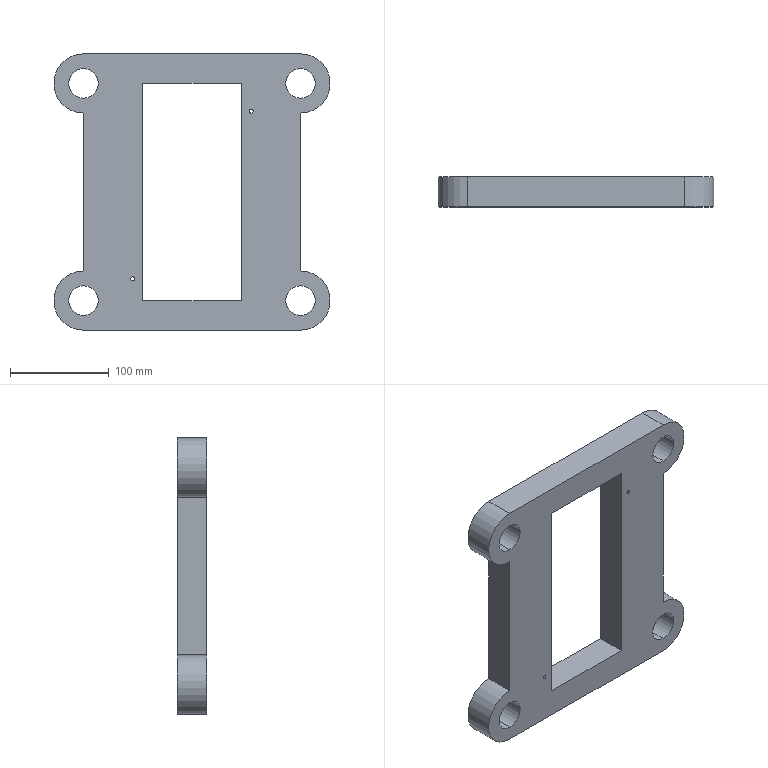Part | SolidWorks | features ICE 2, Extrusion 1, HoleWzd 1, MirrorPattern 1 | 1 solid | 38 faces | box 280 x 30 x 280 mm | volume 1265786 mm3 | cylinder 24 | plane 14 | commonest cylinder face diameters 10 x8 30 x8 4 x4 60 x4
STEP:
#1=CARTESIAN_POINT('',(-60.,0.,19.935));
#2=VERTEX_POINT('',#1);
#3=CARTESIAN_POINT('',(-60.,0.,23.935));
#4=VERTEX_POINT('',#3);
#5=CARTESIAN_POINT('',(-60.,0.,21.935));
#6=DIRECTION('',(0.,1.,0.));
#7=DIRECTION('',(0.,0.,1.));
#8=AXIS2_PLACEMENT_3D('',#5,#6,#7);
#9=CIRCLE('',#8,2.);
#10=EDGE_CURVE('',#2,#4,#9,.T.);
#11=ORIENTED_EDGE('',*,*,#10,.F.);
#12=CARTESIAN_POINT('',(-60.,30.,19.935));
#13=VERTEX_POINT('',#12);
#14=CARTESIAN_POINT('',(-60.,0.,19.935));
#15=DIRECTION('',(0.,1.,0.));
#16=VECTOR('',#15,1000.);
#17=LINE('',#14,#16);
#18=EDGE_CURVE('',#2,#13,#17,.T.);
#19=ORIENTED_EDGE('',*,*,#18,.T.);
#20=CARTESIAN_POINT('',(-60.,30.,23.935));
#21=VERTEX_POINT('',#20);
#22=CARTESIAN_POINT('',(-60.,30.,21.935));
#23=DIRECTION('',(0.,1.,0.));
#24=DIRECTION('',(0.,0.,1.));
#25=AXIS2_PLACEMENT_3D('',#22,#23,#24);
#26=CIRCLE('',#25,2.);
#27=EDGE_CURVE('',#13,#21,#26,.T.);
#28=ORIENTED_EDGE('',*,*,#27,.T.);
#29=CARTESIAN_POINT('',(-60.,0.,23.935));
#30=DIRECTION('',(0.,1.,0.));
#31=VECTOR('',#30,1000.);
#32=LINE('',#29,#31);
#33=EDGE_CURVE('',#4,#21,#32,.T.);
#34=ORIENTED_EDGE('',*,*,#33,.F.);
#35=EDGE_LOOP('',(#11,#19,#28,#34));
#36=FACE_OUTER_BOUND('',#35,.T.);
#37=CARTESIAN_POINT('',(-60.,0.,21.935));
#38=DIRECTION('',(0.,1.,0.));
#39=DIRECTION('',(0.,0.,1.));
#40=AXIS2_PLACEMENT_3D('',#37,#38,#39);
#41=CYLINDRICAL_SURFACE('',#40,2.);
#42=ADVANCED_FACE('',(#36),#41,.F.);
#43=CARTESIAN_POINT('',(60.,0.,189.935));
#44=VERTEX_POINT('',#43);
#45=CARTESIAN_POINT('',(60.,0.,193.935));
#46=VERTEX_POINT('',#45);
#47=CARTESIAN_POINT('',(60.,0.,191.935));
#48=DIRECTION('',(0.,1.,0.));
#49=DIRECTION('',(0.,0.,1.));
#50=AXIS2_PLACEMENT_3D('',#47,#48,#49);
#51=CIRCLE('',#50,2.);
#52=EDGE_CURVE('',#44,#46,#51,.T.);
#53=ORIENTED_EDGE('',*,*,#52,.F.);
#54=CARTESIAN_POINT('',(60.,30.,189.935));
#55=VERTEX_POINT('',#54);
#56=CARTESIAN_POINT('',(60.,0.,189.935));
#57=DIRECTION('',(0.,1.,0.));
#58=VECTOR('',#57,1000.);
#59=LINE('',#56,#58);
#60=EDGE_CURVE('',#44,#55,#59,.T.);
#61=ORIENTED_EDGE('',*,*,#60,.T.);
#62=CARTESIAN_POINT('',(60.,30.,193.935));
#63=VERTEX_POINT('',#62);
#64=CARTESIAN_POINT('',(60.,30.,191.935));
#65=DIRECTION('',(0.,1.,0.));
#66=DIRECTION('',(0.,0.,1.));
#67=AXIS2_PLACEMENT_3D('',#64,#65,#66);
#68=CIRCLE('',#67,2.);
#69=EDGE_CURVE('',#55,#63,#68,.T.);
#70=ORIENTED_EDGE('',*,*,#69,.T.);
#71=CARTESIAN_POINT('',(60.,0.,193.935));
#72=DIRECTION('',(0.,1.,0.));
#73=VECTOR('',#72,1000.);
#74=LINE('',#71,#73);
#75=EDGE_CURVE('',#46,#63,#74,.T.);
#76=ORIENTED_EDGE('',*,*,#75,.F.);
#77=EDGE_LOOP('',(#53,#61,#70,#76));
#78=FACE_OUTER_BOUND('',#77,.T.);
#79=CARTESIAN_POINT('',(60.,0.,191.935));
#80=DIRECTION('',(0.,1.,0.));
#81=DIRECTION('',(0.,0.,1.));
#82=AXIS2_PLACEMENT_3D('',#79,#80,#81);
#83=CYLINDRICAL_SURFACE('',#82,2.);
#84=ADVANCED_FACE('',(#78),#83,.F.);
#85=CARTESIAN_POINT('',(-60.,10.,221.935));
#86=VERTEX_POINT('',#85);
#87=CARTESIAN_POINT('',(-60.,10.,231.935));
#88=VERTEX_POINT('',#87);
#89=CARTESIAN_POINT('',(-60.,10.,226.935));
#90=DIRECTION('',(0.,1.,0.));
#91=DIRECTION('',(0.,0.,1.));
#92=AXIS2_PLACEMENT_3D('',#89,#90,#91);
#93=CIRCLE('',#92,5.);
#94=EDGE_CURVE('',#86,#88,#93,.T.);
#95=ORIENTED_EDGE('',*,*,#94,.F.);
#96=CARTESIAN_POINT('',(-60.,30.,221.935));
#97=VERTEX_POINT('',#96);
#98=CARTESIAN_POINT('',(-60.,10.,221.935));
#99=DIRECTION('',(0.,1.,0.));
#100=VECTOR('',#99,1000.);
#101=LINE('',#98,#100);
#102=EDGE_CURVE('',#86,#97,#101,.T.);
#103=ORIENTED_EDGE('',*,*,#102,.T.);
#104=CARTESIAN_POINT('',(-60.,30.,231.935));
#105=VERTEX_POINT('',#104);
#106=CARTESIAN_POINT('',(-60.,30.,226.935));
#107=DIRECTION('',(0.,1.,0.));
#108=DIRECTION('',(0.,0.,1.));
#109=AXIS2_PLACEMENT_3D('',#106,#107,#108);
#110=CIRCLE('',#109,5.);
#111=EDGE_CURVE('',#97,#105,#110,.T.);
#112=ORIENTED_EDGE('',*,*,#111,.T.);
#113=CARTESIAN_POINT('',(-60.,10.,231.935));
#114=DIRECTION('',(0.,1.,0.));
#115=VECTOR('',#114,1000.);
#116=LINE('',#113,#115);
#117=EDGE_CURVE('',#88,#105,#116,.T.);
#118=ORIENTED_EDGE('',*,*,#117,.F.);
#119=EDGE_LOOP('',(#95,#103,#112,#118));
#120=FACE_OUTER_BOUND('',#119,.T.);
#121=CARTESIAN_POINT('',(-60.,10.,226.935));
#122=DIRECTION('',(0.,1.,0.));
#123=DIRECTION('',(0.,0.,1.));
#124=AXIS2_PLACEMENT_3D('',#121,#122,#123);
#125=CYLINDRICAL_SURFACE('',#124,5.);
#126=ADVANCED_FACE('',(#120),#125,.F.);
#127=CARTESIAN_POINT('',(60.,10.,-18.065));
#128=VERTEX_POINT('',#127);
#129=CARTESIAN_POINT('',(60.,10.,-8.065));
#130=VERTEX_POINT('',#129);
#131=CARTESIAN_POINT('',(60.,10.,-13.065));
#132=DIRECTION('',(0.,1.,0.));
#133=DIRECTION('',(0.,0.,-1.));
#134=AXIS2_PLACEMENT_3D('',#131,#132,#133);
#135=CIRCLE('',#134,5.);
#136=EDGE_CURVE('',#128,#130,#135,.T.);
#137=ORIENTED_EDGE('',*,*,#136,.F.);
#138=CARTESIAN_POINT('',(60.,30.,-18.065));
#139=VERTEX_POINT('',#138);
#140=CARTESIAN_POINT('',(60.,10.,-18.065));
#141=DIRECTION('',(0.,1.,0.));
#142=VECTOR('',#141,1000.);
#143=LINE('',#140,#142);
#144=EDGE_CURVE('',#128,#139,#143,.T.);
#145=ORIENTED_EDGE('',*,*,#144,.T.);
#146=CARTESIAN_POINT('',(60.,30.,-8.065));
#147=VERTEX_POINT('',#146);
#148=CARTESIAN_POINT('',(60.,30.,-13.065));
#149=DIRECTION('',(0.,1.,0.));
#150=DIRECTION('',(0.,0.,-1.));
#151=AXIS2_PLACEMENT_3D('',#148,#149,#150);
#152=CIRCLE('',#151,5.);
#153=EDGE_CURVE('',#139,#147,#152,.T.);
#154=ORIENTED_EDGE('',*,*,#153,.T.);
#155=CARTESIAN_POINT('',(60.,10.,-8.065));
#156=DIRECTION('',(0.,1.,0.));
#157=VECTOR('',#156,1000.);
#158=LINE('',#155,#157);
#159=EDGE_CURVE('',#130,#147,#158,.T.);
#160=ORIENTED_EDGE('',*,*,#159,.F.);
#161=EDGE_LOOP('',(#137,#145,#154,#160));
#162=FACE_OUTER_BOUND('',#161,.T.);
#163=CARTESIAN_POINT('',(60.,10.,-13.065));
#164=DIRECTION('',(0.,1.,0.));
#165=DIRECTION('',(0.,0.,1.));
#166=AXIS2_PLACEMENT_3D('',#163,#164,#165);
#167=CYLINDRICAL_SURFACE('',#166,5.);
#168=ADVANCED_FACE('',(#162),#167,.F.);
#169=CARTESIAN_POINT('',(60.,10.,221.935));
#170=VERTEX_POINT('',#169);
#171=CARTESIAN_POINT('',(60.,10.,231.935));
#172=VERTEX_POINT('',#171);
#173=CARTESIAN_POINT('',(60.,10.,226.935));
#174=DIRECTION('',(0.,1.,0.));
#175=DIRECTION('',(0.,0.,-1.));
#176=AXIS2_PLACEMENT_3D('',#173,#174,#175);
#177=CIRCLE('',#176,5.);
#178=EDGE_CURVE('',#170,#172,#177,.T.);
#179=ORIENTED_EDGE('',*,*,#178,.F.);
#180=CARTESIAN_POINT('',(60.,30.,221.935));
#181=VERTEX_POINT('',#180);
#182=CARTESIAN_POINT('',(60.,10.,221.935));
#183=DIRECTION('',(0.,1.,0.));
#184=VECTOR('',#183,1000.);
#185=LINE('',#182,#184);
#186=EDGE_CURVE('',#170,#181,#185,.T.);
#187=ORIENTED_EDGE('',*,*,#186,.T.);
#188=CARTESIAN_POINT('',(60.,30.,231.935));
#189=VERTEX_POINT('',#188);
#190=CARTESIAN_POINT('',(60.,30.,226.935));
#191=DIRECTION('',(0.,1.,0.));
#192=DIRECTION('',(0.,0.,-1.));
#193=AXIS2_PLACEMENT_3D('',#190,#191,#192);
#194=CIRCLE('',#193,5.);
#195=EDGE_CURVE('',#181,#189,#194,.T.);
#196=ORIENTED_EDGE('',*,*,#195,.T.);
#197=CARTESIAN_POINT('',(60.,10.,231.935));
#198=DIRECTION('',(0.,1.,0.));
#199=VECTOR('',#198,1000.);
#200=LINE('',#197,#199);
#201=EDGE_CURVE('',#172,#189,#200,.T.);
#202=ORIENTED_EDGE('',*,*,#201,.F.);
#203=EDGE_LOOP('',(#179,#187,#196,#202));
#204=FACE_OUTER_BOUND('',#203,.T.);
#205=CARTESIAN_POINT('',(60.,10.,226.935));
#206=DIRECTION('',(0.,1.,0.));
#207=DIRECTION('',(0.,0.,1.));
#208=AXIS2_PLACEMENT_3D('',#205,#206,#207);
#209=CYLINDRICAL_SURFACE('',#208,5.);
#210=ADVANCED_FACE('',(#204),#209,.F.);
#211=CARTESIAN_POINT('',(-60.,10.,-18.065));
#212=VERTEX_POINT('',#211);
#213=CARTESIAN_POINT('',(-60.,10.,-8.065));
#214=VERTEX_POINT('',#213);
#215=CARTESIAN_POINT('',(-60.,10.,-13.065));
#216=DIRECTION('',(0.,1.,0.));
#217=DIRECTION('',(0.,0.,1.));
#218=AXIS2_PLACEMENT_3D('',#215,#216,#217);
#219=CIRCLE('',#218,5.);
#220=EDGE_CURVE('',#212,#214,#219,.T.);
#221=ORIENTED_EDGE('',*,*,#220,.F.);
#222=CARTESIAN_POINT('',(-60.,30.,-18.065));
#223=VERTEX_POINT('',#222);
#224=CARTESIAN_POINT('',(-60.,10.,-18.065));
#225=DIRECTION('',(0.,1.,0.));
#226=VECTOR('',#225,1000.);
#227=LINE('',#224,#226);
#228=EDGE_CURVE('',#212,#223,#227,.T.);
#229=ORIENTED_EDGE('',*,*,#228,.T.);
#230=CARTESIAN_POINT('',(-60.,30.,-8.065));
#231=VERTEX_POINT('',#230);
#232=CARTESIAN_POINT('',(-60.,30.,-13.065));
#233=DIRECTION('',(0.,1.,0.));
#234=DIRECTION('',(0.,0.,1.));
#235=AXIS2_PLACEMENT_3D('',#232,#233,#234);
#236=CIRCLE('',#235,5.);
#237=EDGE_CURVE('',#223,#231,#236,.T.);
#238=ORIENTED_EDGE('',*,*,#237,.T.);
#239=CARTESIAN_POINT('',(-60.,10.,-8.065));
#240=DIRECTION('',(0.,1.,0.));
#241=VECTOR('',#240,1000.);
#242=LINE('',#239,#241);
#243=EDGE_CURVE('',#214,#231,#242,.T.);
#244=ORIENTED_EDGE('',*,*,#243,.F.);
#245=EDGE_LOOP('',(#221,#229,#238,#244));
#246=FACE_OUTER_BOUND('',#245,.T.);
#247=CARTESIAN_POINT('',(-60.,10.,-13.065));
#248=DIRECTION('',(0.,1.,0.));
#249=DIRECTION('',(0.,0.,1.));
#250=AXIS2_PLACEMENT_3D('',#247,#248,#249);
#251=CYLINDRICAL_SURFACE('',#250,5.);
#252=ADVANCED_FACE('',(#246),#251,.F.);
#253=CARTESIAN_POINT('',(110.,30.,235.));
#254=VERTEX_POINT('',#253);
#255=CARTESIAN_POINT('',(110.,30.,205.));
#256=VERTEX_POINT('',#255);
#257=CARTESIAN_POINT('',(110.,30.,220.));
#258=DIRECTION('',(0.,-1.,0.));
#259=DIRECTION('',(0.,0.,1.));
#260=AXIS2_PLACEMENT_3D('',#257,#258,#259);
#261=CIRCLE('',#260,15.);
#262=EDGE_CURVE('',#254,#256,#261,.T.);
#263=ORIENTED_EDGE('',*,*,#262,.F.);
#264=CARTESIAN_POINT('',(110.,0.,235.));
#265=VERTEX_POINT('',#264);
#266=CARTESIAN_POINT('',(110.,30.,235.));
#267=DIRECTION('',(0.,-1.,0.));
#268=VECTOR('',#267,1000.);
#269=LINE('',#266,#268);
#270=EDGE_CURVE('',#254,#265,#269,.T.);
#271=ORIENTED_EDGE('',*,*,#270,.T.);
#272=CARTESIAN_POINT('',(110.,0.,205.));
#273=VERTEX_POINT('',#272);
#274=CARTESIAN_POINT('',(110.,0.,220.));
#275=DIRECTION('',(0.,-1.,0.));
#276=DIRECTION('',(0.,0.,1.));
#277=AXIS2_PLACEMENT_3D('',#274,#275,#276);
#278=CIRCLE('',#277,15.);
#279=EDGE_CURVE('',#265,#273,#278,.T.);
#280=ORIENTED_EDGE('',*,*,#279,.T.);
#281=CARTESIAN_POINT('',(110.,30.,205.));
#282=DIRECTION('',(0.,-1.,0.));
#283=VECTOR('',#282,1000.);
#284=LINE('',#281,#283);
#285=EDGE_CURVE('',#256,#273,#284,.T.);
#286=ORIENTED_EDGE('',*,*,#285,.F.);
#287=EDGE_LOOP('',(#263,#271,#280,#286));
#288=FACE_OUTER_BOUND('',#287,.T.);
#289=CARTESIAN_POINT('',(110.,30.,220.));
#290=DIRECTION('',(0.,-1.,0.));
#291=DIRECTION('',(0.,0.,-1.));
#292=AXIS2_PLACEMENT_3D('',#289,#290,#291);
#293=CYLINDRICAL_SURFACE('',#292,15.);
#294=ADVANCED_FACE('',(#288),#293,.F.);
#295=CARTESIAN_POINT('',(110.,30.,15.));
#296=VERTEX_POINT('',#295);
#297=CARTESIAN_POINT('',(110.,30.,-15.));
#298=VERTEX_POINT('',#297);
#299=CARTESIAN_POINT('',(110.,30.,0.));
#300=DIRECTION('',(0.,-1.,0.));
#301=DIRECTION('',(0.,0.,1.));
#302=AXIS2_PLACEMENT_3D('',#299,#300,#301);
#303=CIRCLE('',#302,15.);
#304=EDGE_CURVE('',#296,#298,#303,.T.);
#305=ORIENTED_EDGE('',*,*,#304,.F.);
#306=CARTESIAN_POINT('',(110.,0.,15.));
#307=VERTEX_POINT('',#306);
#308=CARTESIAN_POINT('',(110.,30.,15.));
#309=DIRECTION('',(0.,-1.,0.));
#310=VECTOR('',#309,1000.);
#311=LINE('',#308,#310);
#312=EDGE_CURVE('',#296,#307,#311,.T.);
#313=ORIENTED_EDGE('',*,*,#312,.T.);
#314=CARTESIAN_POINT('',(110.,0.,-15.));
#315=VERTEX_POINT('',#314);
#316=CARTESIAN_POINT('',(110.,0.,0.));
#317=DIRECTION('',(0.,-1.,0.));
#318=DIRECTION('',(0.,0.,1.));
#319=AXIS2_PLACEMENT_3D('',#316,#317,#318);
#320=CIRCLE('',#319,15.);
#321=EDGE_CURVE('',#307,#315,#320,.T.);
#322=ORIENTED_EDGE('',*,*,#321,.T.);
#323=CARTESIAN_POINT('',(110.,30.,-15.));
#324=DIRECTION('',(0.,-1.,0.));
#325=VECTOR('',#324,1000.);
#326=LINE('',#323,#325);
#327=EDGE_CURVE('',#298,#315,#326,.T.);
#328=ORIENTED_EDGE('',*,*,#327,.F.);
#329=EDGE_LOOP('',(#305,#313,#322,#328));
#330=FACE_OUTER_BOUND('',#329,.T.);
#331=CARTESIAN_POINT('',(110.,30.,0.));
#332=DIRECTION('',(0.,-1.,0.));
#333=DIRECTION('',(0.,0.,-1.));
#334=AXIS2_PLACEMENT_3D('',#331,#332,#333);
#335=CYLINDRICAL_SURFACE('',#334,15.);
#336=ADVANCED_FACE('',(#330),#335,.F.);
#337=CARTESIAN_POINT('',(-110.,30.,205.));
#338=VERTEX_POINT('',#337);
#339=CARTESIAN_POINT('',(-110.,30.,235.));
#340=VERTEX_POINT('',#339);
#341=CARTESIAN_POINT('',(-110.,30.,220.));
#342=DIRECTION('',(0.,1.,0.));
#343=DIRECTION('',(0.,0.,1.));
#344=AXIS2_PLACEMENT_3D('',#341,#342,#343);
#345=CIRCLE('',#344,15.);
#346=EDGE_CURVE('',#338,#340,#345,.T.);
#347=ORIENTED_EDGE('',*,*,#346,.T.);
#348=CARTESIAN_POINT('',(-110.,0.,235.));
#349=VERTEX_POINT('',#348);
#350=CARTESIAN_POINT('',(-110.,30.,235.));
#351=DIRECTION('',(0.,-1.,0.));
#352=VECTOR('',#351,1000.);
#353=LINE('',#350,#352);
#354=EDGE_CURVE('',#340,#349,#353,.T.);
#355=ORIENTED_EDGE('',*,*,#354,.T.);
#356=CARTESIAN_POINT('',(-110.,0.,205.));
#357=VERTEX_POINT('',#356);
#358=CARTESIAN_POINT('',(-110.,0.,220.));
#359=DIRECTION('',(0.,1.,0.));
#360=DIRECTION('',(0.,0.,1.));
#361=AXIS2_PLACEMENT_3D('',#358,#359,#360);
#362=CIRCLE('',#361,15.);
#363=EDGE_CURVE('',#357,#349,#362,.T.);
#364=ORIENTED_EDGE('',*,*,#363,.F.);
#365=CARTESIAN_POINT('',(-110.,30.,205.));
#366=DIRECTION('',(0.,-1.,0.));
#367=VECTOR('',#366,1000.);
#368=LINE('',#365,#367);
#369=EDGE_CURVE('',#338,#357,#368,.T.);
#370=ORIENTED_EDGE('',*,*,#369,.F.);
#371=EDGE_LOOP('',(#347,#355,#364,#370));
#372=FACE_OUTER_BOUND('',#371,.T.);
#373=CARTESIAN_POINT('',(-110.,30.,220.));
#374=DIRECTION('',(0.,-1.,0.));
#375=DIRECTION('',(0.,0.,-1.));
#376=AXIS2_PLACEMENT_3D('',#373,#374,#375);
#377=CYLINDRICAL_SURFACE('',#376,15.);
#378=ADVANCED_FACE('',(#372),#377,.F.);
#379=CARTESIAN_POINT('',(-110.,30.,-15.));
#380=VERTEX_POINT('',#379);
#381=CARTESIAN_POINT('',(-110.,30.,15.));
#382=VERTEX_POINT('',#381);
#383=CARTESIAN_POINT('',(-110.,30.,0.));
#384=DIRECTION('',(0.,1.,0.));
#385=DIRECTION('',(0.,0.,1.));
#386=AXIS2_PLACEMENT_3D('',#383,#384,#385);
#387=CIRCLE('',#386,15.);
#388=EDGE_CURVE('',#380,#382,#387,.T.);
#389=ORIENTED_EDGE('',*,*,#388,.T.);
#390=CARTESIAN_POINT('',(-110.,0.,15.));
#391=VERTEX_POINT('',#390);
#392=CARTESIAN_POINT('',(-110.,30.,15.));
#393=DIRECTION('',(0.,-1.,0.));
#394=VECTOR('',#393,1000.);
#395=LINE('',#392,#394);
#396=EDGE_CURVE('',#382,#391,#395,.T.);
#397=ORIENTED_EDGE('',*,*,#396,.T.);
#398=CARTESIAN_POINT('',(-110.,0.,-15.));
#399=VERTEX_POINT('',#398);
#400=CARTESIAN_POINT('',(-110.,0.,0.));
#401=DIRECTION('',(0.,1.,0.));
#402=DIRECTION('',(0.,0.,1.));
#403=AXIS2_PLACEMENT_3D('',#400,#401,#402);
#404=CIRCLE('',#403,15.);
#405=EDGE_CURVE('',#399,#391,#404,.T.);
#406=ORIENTED_EDGE('',*,*,#405,.F.);
#407=CARTESIAN_POINT('',(-110.,30.,-15.));
#408=DIRECTION('',(0.,-1.,0.));
#409=VECTOR('',#408,1000.);
#410=LINE('',#407,#409);
#411=EDGE_CURVE('',#380,#399,#410,.T.);
#412=ORIENTED_EDGE('',*,*,#411,.F.);
#413=EDGE_LOOP('',(#389,#397,#406,#412));
#414=FACE_OUTER_BOUND('',#413,.T.);
#415=CARTESIAN_POINT('',(-110.,30.,0.));
#416=DIRECTION('',(0.,-1.,0.));
#417=DIRECTION('',(0.,0.,-1.));
#418=AXIS2_PLACEMENT_3D('',#415,#416,#417);
#419=CYLINDRICAL_SURFACE('',#418,15.);
#420=ADVANCED_FACE('',(#414),#419,.F.);
#421=CARTESIAN_POINT('',(-60.,30.,21.935));
#422=DIRECTION('',(0.,1.,0.));
#423=DIRECTION('',(0.,0.,1.));
#424=AXIS2_PLACEMENT_3D('',#421,#422,#423);
#425=CIRCLE('',#424,2.);
#426=EDGE_CURVE('',#21,#13,#425,.T.);
#427=ORIENTED_EDGE('',*,*,#426,.F.);
#428=ORIENTED_EDGE('',*,*,#27,.F.);
#429=EDGE_LOOP('',(#427,#428));
#430=FACE_BOUND('',#429,.T.);
#431=CARTESIAN_POINT('',(60.,30.,191.935));
#432=DIRECTION('',(0.,1.,0.));
#433=DIRECTION('',(0.,0.,1.));
#434=AXIS2_PLACEMENT_3D('',#431,#432,#433);
#435=CIRCLE('',#434,2.);
#436=EDGE_CURVE('',#63,#55,#435,.T.);
#437=ORIENTED_EDGE('',*,*,#436,.F.);
#438=ORIENTED_EDGE('',*,*,#69,.F.);
#439=EDGE_LOOP('',(#437,#438));
#440=FACE_BOUND('',#439,.T.);
#441=CARTESIAN_POINT('',(-60.,30.,226.935));
#442=DIRECTION('',(0.,1.,0.));
#443=DIRECTION('',(0.,0.,1.));
#444=AXIS2_PLACEMENT_3D('',#441,#442,#443);
#445=CIRCLE('',#444,5.);
#446=EDGE_CURVE('',#105,#97,#445,.T.);
#447=ORIENTED_EDGE('',*,*,#446,.F.);
#448=ORIENTED_EDGE('',*,*,#111,.F.);
#449=EDGE_LOOP('',(#447,#448));
#450=FACE_BOUND('',#449,.T.);
#451=CARTESIAN_POINT('',(60.,30.,-13.065));
#452=DIRECTION('',(0.,1.,0.));
#453=DIRECTION('',(0.,0.,-1.));
#454=AXIS2_PLACEMENT_3D('',#451,#452,#453);
#455=CIRCLE('',#454,5.);
#456=EDGE_CURVE('',#147,#139,#455,.T.);
#457=ORIENTED_EDGE('',*,*,#456,.F.);
#458=ORIENTED_EDGE('',*,*,#153,.F.);
#459=EDGE_LOOP('',(#457,#458));
#460=FACE_BOUND('',#459,.T.);
#461=CARTESIAN_POINT('',(60.,30.,226.935));
#462=DIRECTION('',(0.,1.,0.));
#463=DIRECTION('',(0.,0.,-1.));
#464=AXIS2_PLACEMENT_3D('',#461,#462,#463);
#465=CIRCLE('',#464,5.);
#466=EDGE_CURVE('',#189,#181,#465,.T.);
#467=ORIENTED_EDGE('',*,*,#466,.F.);
#468=ORIENTED_EDGE('',*,*,#195,.F.);
#469=EDGE_LOOP('',(#467,#468));
#470=FACE_BOUND('',#469,.T.);
#471=CARTESIAN_POINT('',(-60.,30.,-13.065));
#472=DIRECTION('',(0.,1.,0.));
#473=DIRECTION('',(0.,0.,1.));
#474=AXIS2_PLACEMENT_3D('',#471,#472,#473);
#475=CIRCLE('',#474,5.);
#476=EDGE_CURVE('',#231,#223,#475,.T.);
#477=ORIENTED_EDGE('',*,*,#476,.F.);
#478=ORIENTED_EDGE('',*,*,#237,.F.);
#479=EDGE_LOOP('',(#477,#478));
#480=FACE_BOUND('',#479,.T.);
#481=CARTESIAN_POINT('',(-110.,30.,250.));
#482=VERTEX_POINT('',#481);
#483=CARTESIAN_POINT('',(110.,30.,250.));
#484=VERTEX_POINT('',#483);
#485=CARTESIAN_POINT('',(-110.,30.,250.));
#486=DIRECTION('',(1.,0.,0.));
#487=VECTOR('',#486,1000.);
#488=LINE('',#485,#487);
#489=EDGE_CURVE('',#482,#484,#488,.T.);
#490=ORIENTED_EDGE('',*,*,#489,.T.);
#491=CARTESIAN_POINT('',(110.,30.,190.));
#492=VERTEX_POINT('',#491);
#493=CARTESIAN_POINT('',(110.,30.,220.));
#494=DIRECTION('',(0.,-1.,0.));
#495=DIRECTION('',(0.,0.,1.));
#496=AXIS2_PLACEMENT_3D('',#493,#494,#495);
#497=CIRCLE('',#496,30.);
#498=EDGE_CURVE('',#492,#484,#497,.T.);
#499=ORIENTED_EDGE('',*,*,#498,.F.);
#500=CARTESIAN_POINT('',(110.,30.,30.));
#501=VERTEX_POINT('',#500);
#502=CARTESIAN_POINT('',(110.,30.,190.));
#503=DIRECTION('',(0.,0.,1.));
#504=VECTOR('',#503,1000.);
#505=LINE('',#502,#504);
#506=EDGE_CURVE('',#501,#492,#505,.T.);
#507=ORIENTED_EDGE('',*,*,#506,.F.);
#508=CARTESIAN_POINT('',(110.,30.,-30.));
#509=VERTEX_POINT('',#508);
#510=CARTESIAN_POINT('',(110.,30.,0.));
#511=DIRECTION('',(0.,-1.,0.));
#512=DIRECTION('',(0.,0.,1.));
#513=AXIS2_PLACEMENT_3D('',#510,#511,#512);
#514=CIRCLE('',#513,30.);
#515=EDGE_CURVE('',#509,#501,#514,.T.);
#516=ORIENTED_EDGE('',*,*,#515,.F.);
#517=CARTESIAN_POINT('',(-110.,30.,-30.));
#518=VERTEX_POINT('',#517);
#519=CARTESIAN_POINT('',(80.,30.,-30.));
#520=DIRECTION('',(-1.,0.,0.));
#521=VECTOR('',#520,1000.);
#522=LINE('',#519,#521);
#523=EDGE_CURVE('',#509,#518,#522,.T.);
#524=ORIENTED_EDGE('',*,*,#523,.T.);
#525=CARTESIAN_POINT('',(-110.,30.,30.));
#526=VERTEX_POINT('',#525);
#527=CARTESIAN_POINT('',(-110.,30.,0.));
#528=DIRECTION('',(0.,1.,0.));
#529=DIRECTION('',(0.,0.,1.));
#530=AXIS2_PLACEMENT_3D('',#527,#528,#529);
#531=CIRCLE('',#530,30.);
#532=EDGE_CURVE('',#518,#526,#531,.T.);
#533=ORIENTED_EDGE('',*,*,#532,.T.);
#534=CARTESIAN_POINT('',(-110.,30.,190.));
#535=VERTEX_POINT('',#534);
#536=CARTESIAN_POINT('',(-110.,30.,190.));
#537=DIRECTION('',(0.,0.,1.));
#538=VECTOR('',#537,1000.);
#539=LINE('',#536,#538);
#540=EDGE_CURVE('',#526,#535,#539,.T.);
#541=ORIENTED_EDGE('',*,*,#540,.T.);
#542=CARTESIAN_POINT('',(-110.,30.,220.));
#543=DIRECTION('',(0.,1.,0.));
#544=DIRECTION('',(0.,0.,1.));
#545=AXIS2_PLACEMENT_3D('',#542,#543,#544);
#546=CIRCLE('',#545,30.);
#547=EDGE_CURVE('',#535,#482,#546,.T.);
#548=ORIENTED_EDGE('',*,*,#547,.T.);
#549=EDGE_LOOP('',(#490,#499,#507,#516,#524,#533,#541,#548));
#550=FACE_OUTER_BOUND('',#549,.T.);
#551=ORIENTED_EDGE('',*,*,#388,.F.);
#552=CARTESIAN_POINT('',(-110.,30.,0.));
#553=DIRECTION('',(0.,1.,0.));
#554=DIRECTION('',(0.,0.,1.));
#555=AXIS2_PLACEMENT_3D('',#552,#553,#554);
#556=CIRCLE('',#555,15.);
#557=EDGE_CURVE('',#382,#380,#556,.T.);
#558=ORIENTED_EDGE('',*,*,#557,.F.);
#559=EDGE_LOOP('',(#551,#558));
#560=FACE_BOUND('',#559,.T.);
#561=ORIENTED_EDGE('',*,*,#346,.F.);
#562=CARTESIAN_POINT('',(-110.,30.,220.));
#563=DIRECTION('',(0.,1.,0.));
#564=DIRECTION('',(0.,0.,1.));
#565=AXIS2_PLACEMENT_3D('',#562,#563,#564);
#566=CIRCLE('',#565,15.);
#567=EDGE_CURVE('',#340,#338,#566,.T.);
#568=ORIENTED_EDGE('',*,*,#567,.F.);
#569=EDGE_LOOP('',(#561,#568));
#570=FACE_BOUND('',#569,.T.);
#571=CARTESIAN_POINT('',(-50.,30.,0.));
#572=VERTEX_POINT('',#571);
#573=CARTESIAN_POINT('',(-50.,30.,220.));
#574=VERTEX_POINT('',#573);
#575=CARTESIAN_POINT('',(-50.,30.,0.));
#576=DIRECTION('',(0.,0.,1.));
#577=VECTOR('',#576,1000.);
#578=LINE('',#575,#577);
#579=EDGE_CURVE('',#572,#574,#578,.T.);
#580=ORIENTED_EDGE('',*,*,#579,.F.);
#581=CARTESIAN_POINT('',(50.,30.,0.));
#582=VERTEX_POINT('',#581);
#583=CARTESIAN_POINT('',(50.,30.,0.));
#584=DIRECTION('',(-1.,0.,0.));
#585=VECTOR('',#584,1000.);
#586=LINE('',#583,#585);
#587=EDGE_CURVE('',#582,#572,#586,.T.);
#588=ORIENTED_EDGE('',*,*,#587,.F.);
#589=CARTESIAN_POINT('',(50.,30.,220.));
#590=VERTEX_POINT('',#589);
#591=CARTESIAN_POINT('',(50.,30.,220.));
#592=DIRECTION('',(0.,0.,-1.));
#593=VECTOR('',#592,1000.);
#594=LINE('',#591,#593);
#595=EDGE_CURVE('',#590,#582,#594,.T.);
#596=ORIENTED_EDGE('',*,*,#595,.F.);
#597=CARTESIAN_POINT('',(-50.,30.,220.));
#598=DIRECTION('',(1.,0.,0.));
#599=VECTOR('',#598,1000.);
#600=LINE('',#597,#599);
#601=EDGE_CURVE('',#574,#590,#600,.T.);
#602=ORIENTED_EDGE('',*,*,#601,.F.);
#603=EDGE_LOOP('',(#580,#588,#596,#602));
#604=FACE_BOUND('',#603,.T.);
#605=CARTESIAN_POINT('',(110.,30.,0.));
#606=DIRECTION('',(0.,-1.,0.));
#607=DIRECTION('',(0.,0.,1.));
#608=AXIS2_PLACEMENT_3D('',#605,#606,#607);
#609=CIRCLE('',#608,15.);
#610=EDGE_CURVE('',#298,#296,#609,.T.);
#611=ORIENTED_EDGE('',*,*,#610,.T.);
#612=ORIENTED_EDGE('',*,*,#304,.T.);
#613=EDGE_LOOP('',(#611,#612));
#614=FACE_BOUND('',#613,.T.);
#615=CARTESIAN_POINT('',(110.,30.,220.));
#616=DIRECTION('',(0.,-1.,0.));
#617=DIRECTION('',(0.,0.,1.));
#618=AXIS2_PLACEMENT_3D('',#615,#616,#617);
#619=CIRCLE('',#618,15.);
#620=EDGE_CURVE('',#256,#254,#619,.T.);
#621=ORIENTED_EDGE('',*,*,#620,.T.);
#622=ORIENTED_EDGE('',*,*,#262,.T.);
#623=EDGE_LOOP('',(#621,#622));
#624=FACE_BOUND('',#623,.T.);
#625=CARTESIAN_POINT('',(-110.,30.,0.));
#626=DIRECTION('',(0.,1.,0.));
#627=DIRECTION('',(0.,0.,1.));
#628=AXIS2_PLACEMENT_3D('',#625,#626,#627);
#629=PLANE('',#628);
#630=ADVANCED_FACE('',(#430,#440,#450,#460,#470,#480,#550,#560,#570,#604,#614,#624),#629,.T.);
#631=CARTESIAN_POINT('',(-60.,0.,21.935));
#632=DIRECTION('',(0.,1.,0.));
#633=DIRECTION('',(0.,0.,1.));
#634=AXIS2_PLACEMENT_3D('',#631,#632,#633);
#635=CIRCLE('',#634,2.);
#636=EDGE_CURVE('',#4,#2,#635,.T.);
#637=ORIENTED_EDGE('',*,*,#636,.T.);
#638=ORIENTED_EDGE('',*,*,#10,.T.);
#639=EDGE_LOOP('',(#637,#638));
#640=FACE_BOUND('',#639,.T.);
#641=CARTESIAN_POINT('',(60.,0.,191.935));
#642=DIRECTION('',(0.,1.,0.));
#643=DIRECTION('',(0.,0.,1.));
#644=AXIS2_PLACEMENT_3D('',#641,#642,#643);
#645=CIRCLE('',#644,2.);
#646=EDGE_CURVE('',#46,#44,#645,.T.);
#647=ORIENTED_EDGE('',*,*,#646,.T.);
#648=ORIENTED_EDGE('',*,*,#52,.T.);
#649=EDGE_LOOP('',(#647,#648));
#650=FACE_BOUND('',#649,.T.);
#651=ORIENTED_EDGE('',*,*,#405,.T.);
#652=CARTESIAN_POINT('',(-110.,0.,0.));
#653=DIRECTION('',(0.,1.,0.));
#654=DIRECTION('',(0.,0.,1.));
#655=AXIS2_PLACEMENT_3D('',#652,#653,#654);
#656=CIRCLE('',#655,15.);
#657=EDGE_CURVE('',#391,#399,#656,.T.);
#658=ORIENTED_EDGE('',*,*,#657,.T.);
#659=EDGE_LOOP('',(#651,#658));
#660=FACE_BOUND('',#659,.T.);
#661=CARTESIAN_POINT('',(-110.,0.,-30.));
#662=VERTEX_POINT('',#661);
#663=CARTESIAN_POINT('',(-110.,0.,30.));
#664=VERTEX_POINT('',#663);
#665=CARTESIAN_POINT('',(-110.,0.,0.));
#666=DIRECTION('',(0.,1.,0.));
#667=DIRECTION('',(0.,0.,1.));
#668=AXIS2_PLACEMENT_3D('',#665,#666,#667);
#669=CIRCLE('',#668,30.);
#670=EDGE_CURVE('',#662,#664,#669,.T.);
#671=ORIENTED_EDGE('',*,*,#670,.F.);
#672=CARTESIAN_POINT('',(110.,0.,-30.));
#673=VERTEX_POINT('',#672);
#674=CARTESIAN_POINT('',(80.,0.,-30.));
#675=DIRECTION('',(-1.,0.,0.));
#676=VECTOR('',#675,1000.);
#677=LINE('',#674,#676);
#678=EDGE_CURVE('',#673,#662,#677,.T.);
#679=ORIENTED_EDGE('',*,*,#678,.F.);
#680=CARTESIAN_POINT('',(110.,0.,30.));
#681=VERTEX_POINT('',#680);
#682=CARTESIAN_POINT('',(110.,0.,0.));
#683=DIRECTION('',(0.,-1.,0.));
#684=DIRECTION('',(0.,0.,1.));
#685=AXIS2_PLACEMENT_3D('',#682,#683,#684);
#686=CIRCLE('',#685,30.);
#687=EDGE_CURVE('',#673,#681,#686,.T.);
#688=ORIENTED_EDGE('',*,*,#687,.T.);
#689=CARTESIAN_POINT('',(110.,0.,190.));
#690=VERTEX_POINT('',#689);
#691=CARTESIAN_POINT('',(110.,0.,190.));
#692=DIRECTION('',(0.,0.,1.));
#693=VECTOR('',#692,1000.);
#694=LINE('',#691,#693);
#695=EDGE_CURVE('',#681,#690,#694,.T.);
#696=ORIENTED_EDGE('',*,*,#695,.T.);
#697=CARTESIAN_POINT('',(110.,0.,250.));
#698=VERTEX_POINT('',#697);
#699=CARTESIAN_POINT('',(110.,0.,220.));
#700=DIRECTION('',(0.,-1.,0.));
#701=DIRECTION('',(0.,0.,1.));
#702=AXIS2_PLACEMENT_3D('',#699,#700,#701);
#703=CIRCLE('',#702,30.);
#704=EDGE_CURVE('',#690,#698,#703,.T.);
#705=ORIENTED_EDGE('',*,*,#704,.T.);
#706=CARTESIAN_POINT('',(-110.,0.,250.));
#707=VERTEX_POINT('',#706);
#708=CARTESIAN_POINT('',(-110.,0.,250.));
#709=DIRECTION('',(1.,0.,0.));
#710=VECTOR('',#709,1000.);
#711=LINE('',#708,#710);
#712=EDGE_CURVE('',#707,#698,#711,.T.);
#713=ORIENTED_EDGE('',*,*,#712,.F.);
#714=CARTESIAN_POINT('',(-110.,0.,190.));
#715=VERTEX_POINT('',#714);
#716=CARTESIAN_POINT('',(-110.,0.,220.));
#717=DIRECTION('',(0.,1.,0.));
#718=DIRECTION('',(0.,0.,1.));
#719=AXIS2_PLACEMENT_3D('',#716,#717,#718);
#720=CIRCLE('',#719,30.);
#721=EDGE_CURVE('',#715,#707,#720,.T.);
#722=ORIENTED_EDGE('',*,*,#721,.F.);
#723=CARTESIAN_POINT('',(-110.,0.,190.));
#724=DIRECTION('',(0.,0.,1.));
#725=VECTOR('',#724,1000.);
#726=LINE('',#723,#725);
#727=EDGE_CURVE('',#664,#715,#726,.T.);
#728=ORIENTED_EDGE('',*,*,#727,.F.);
#729=EDGE_LOOP('',(#671,#679,#688,#696,#705,#713,#722,#728));
#730=FACE_OUTER_BOUND('',#729,.T.);
#731=ORIENTED_EDGE('',*,*,#363,.T.);
#732=CARTESIAN_POINT('',(-110.,0.,220.));
#733=DIRECTION('',(0.,1.,0.));
#734=DIRECTION('',(0.,0.,1.));
#735=AXIS2_PLACEMENT_3D('',#732,#733,#734);
#736=CIRCLE('',#735,15.);
#737=EDGE_CURVE('',#349,#357,#736,.T.);
#738=ORIENTED_EDGE('',*,*,#737,.T.);
#739=EDGE_LOOP('',(#731,#738));
#740=FACE_BOUND('',#739,.T.);
#741=CARTESIAN_POINT('',(50.,0.,0.));
#742=VERTEX_POINT('',#741);
#743=CARTESIAN_POINT('',(-50.,0.,0.));
#744=VERTEX_POINT('',#743);
#745=CARTESIAN_POINT('',(50.,0.,0.));
#746=DIRECTION('',(-1.,0.,0.));
#747=VECTOR('',#746,1000.);
#748=LINE('',#745,#747);
#749=EDGE_CURVE('',#742,#744,#748,.T.);
#750=ORIENTED_EDGE('',*,*,#749,.T.);
#751=CARTESIAN_POINT('',(-50.,0.,220.));
#752=VERTEX_POINT('',#751);
#753=CARTESIAN_POINT('',(-50.,0.,0.));
#754=DIRECTION('',(0.,0.,1.));
#755=VECTOR('',#754,1000.);
#756=LINE('',#753,#755);
#757=EDGE_CURVE('',#744,#752,#756,.T.);
#758=ORIENTED_EDGE('',*,*,#757,.T.);
#759=CARTESIAN_POINT('',(50.,0.,220.));
#760=VERTEX_POINT('',#759);
#761=CARTESIAN_POINT('',(-50.,0.,220.));
#762=DIRECTION('',(1.,0.,0.));
#763=VECTOR('',#762,1000.);
#764=LINE('',#761,#763);
#765=EDGE_CURVE('',#752,#760,#764,.T.);
#766=ORIENTED_EDGE('',*,*,#765,.T.);
#767=CARTESIAN_POINT('',(50.,0.,220.));
#768=DIRECTION('',(0.,0.,-1.));
#769=VECTOR('',#768,1000.);
#770=LINE('',#767,#769);
#771=EDGE_CURVE('',#760,#742,#770,.T.);
#772=ORIENTED_EDGE('',*,*,#771,.T.);
#773=EDGE_LOOP('',(#750,#758,#766,#772));
#774=FACE_BOUND('',#773,.T.);
#775=CARTESIAN_POINT('',(110.,0.,0.));
#776=DIRECTION('',(0.,-1.,0.));
#777=DIRECTION('',(0.,0.,1.));
#778=AXIS2_PLACEMENT_3D('',#775,#776,#777);
#779=CIRCLE('',#778,15.);
#780=EDGE_CURVE('',#315,#307,#779,.T.);
#781=ORIENTED_EDGE('',*,*,#780,.F.);
#782=ORIENTED_EDGE('',*,*,#321,.F.);
#783=EDGE_LOOP('',(#781,#782));
#784=FACE_BOUND('',#783,.T.);
#785=CARTESIAN_POINT('',(110.,0.,220.));
#786=DIRECTION('',(0.,-1.,0.));
#787=DIRECTION('',(0.,0.,1.));
#788=AXIS2_PLACEMENT_3D('',#785,#786,#787);
#789=CIRCLE('',#788,15.);
#790=EDGE_CURVE('',#273,#265,#789,.T.);
#791=ORIENTED_EDGE('',*,*,#790,.F.);
#792=ORIENTED_EDGE('',*,*,#279,.F.);
#793=EDGE_LOOP('',(#791,#792));
#794=FACE_BOUND('',#793,.T.);
#795=CARTESIAN_POINT('',(-110.,0.,0.));
#796=DIRECTION('',(0.,1.,0.));
#797=DIRECTION('',(0.,0.,1.));
#798=AXIS2_PLACEMENT_3D('',#795,#796,#797);
#799=PLANE('',#798);
#800=ADVANCED_FACE('',(#640,#650,#660,#730,#740,#774,#784,#794),#799,.F.);
#801=ORIENTED_EDGE('',*,*,#670,.T.);
#802=CARTESIAN_POINT('',(-110.,30.,30.));
#803=DIRECTION('',(0.,-1.,0.));
#804=VECTOR('',#803,1000.);
#805=LINE('',#802,#804);
#806=EDGE_CURVE('',#526,#664,#805,.T.);
#807=ORIENTED_EDGE('',*,*,#806,.F.);
#808=ORIENTED_EDGE('',*,*,#532,.F.);
#809=CARTESIAN_POINT('',(-110.,30.,-30.));
#810=DIRECTION('',(0.,-1.,0.));
#811=VECTOR('',#810,1000.);
#812=LINE('',#809,#811);
#813=EDGE_CURVE('',#518,#662,#812,.T.);
#814=ORIENTED_EDGE('',*,*,#813,.T.);
#815=EDGE_LOOP('',(#801,#807,#808,#814));
#816=FACE_OUTER_BOUND('',#815,.T.);
#817=CARTESIAN_POINT('',(-110.,30.,0.));
#818=DIRECTION('',(0.,-1.,0.));
#819=DIRECTION('',(0.,0.,-1.));
#820=AXIS2_PLACEMENT_3D('',#817,#818,#819);
#821=CYLINDRICAL_SURFACE('',#820,30.);
#822=ADVANCED_FACE('',(#816),#821,.T.);
#823=ORIENTED_EDGE('',*,*,#727,.T.);
#824=CARTESIAN_POINT('',(-110.,30.,190.));
#825=DIRECTION('',(0.,-1.,0.));
#826=VECTOR('',#825,1000.);
#827=LINE('',#824,#826);
#828=EDGE_CURVE('',#535,#715,#827,.T.);
#829=ORIENTED_EDGE('',*,*,#828,.F.);
#830=ORIENTED_EDGE('',*,*,#540,.F.);
#831=ORIENTED_EDGE('',*,*,#806,.T.);
#832=EDGE_LOOP('',(#823,#829,#830,#831));
#833=FACE_OUTER_BOUND('',#832,.T.);
#834=CARTESIAN_POINT('',(-110.,30.,190.));
#835=DIRECTION('',(1.,0.,0.));
#836=DIRECTION('',(0.,0.,-1.));
#837=AXIS2_PLACEMENT_3D('',#834,#835,#836);
#838=PLANE('',#837);
#839=ADVANCED_FACE('',(#833),#838,.F.);
#840=ORIENTED_EDGE('',*,*,#721,.T.);
#841=CARTESIAN_POINT('',(-110.,30.,250.));
#842=DIRECTION('',(0.,-1.,0.));
#843=VECTOR('',#842,1000.);
#844=LINE('',#841,#843);
#845=EDGE_CURVE('',#482,#707,#844,.T.);
#846=ORIENTED_EDGE('',*,*,#845,.F.);
#847=ORIENTED_EDGE('',*,*,#547,.F.);
#848=ORIENTED_EDGE('',*,*,#828,.T.);
#849=EDGE_LOOP('',(#840,#846,#847,#848));
#850=FACE_OUTER_BOUND('',#849,.T.);
#851=CARTESIAN_POINT('',(-110.,30.,220.));
#852=DIRECTION('',(0.,-1.,0.));
#853=DIRECTION('',(0.,0.,-1.));
#854=AXIS2_PLACEMENT_3D('',#851,#852,#853);
#855=CYLINDRICAL_SURFACE('',#854,30.);
#856=ADVANCED_FACE('',(#850),#855,.T.);
#857=ORIENTED_EDGE('',*,*,#712,.T.);
#858=CARTESIAN_POINT('',(110.,30.,250.));
#859=DIRECTION('',(0.,-1.,0.));
#860=VECTOR('',#859,1000.);
#861=LINE('',#858,#860);
#862=EDGE_CURVE('',#484,#698,#861,.T.);
#863=ORIENTED_EDGE('',*,*,#862,.F.);
#864=ORIENTED_EDGE('',*,*,#489,.F.);
#865=ORIENTED_EDGE('',*,*,#845,.T.);
#866=EDGE_LOOP('',(#857,#863,#864,#865));
#867=FACE_OUTER_BOUND('',#866,.T.);
#868=CARTESIAN_POINT('',(-110.,30.,250.));
#869=DIRECTION('',(0.,0.,-1.));
#870=DIRECTION('',(-1.,0.,0.));
#871=AXIS2_PLACEMENT_3D('',#868,#869,#870);
#872=PLANE('',#871);
#873=ADVANCED_FACE('',(#867),#872,.F.);
#874=ORIENTED_EDGE('',*,*,#813,.F.);
#875=ORIENTED_EDGE('',*,*,#523,.F.);
#876=CARTESIAN_POINT('',(110.,30.,-30.));
#877=DIRECTION('',(0.,-1.,0.));
#878=VECTOR('',#877,1000.);
#879=LINE('',#876,#878);
#880=EDGE_CURVE('',#509,#673,#879,.T.);
#881=ORIENTED_EDGE('',*,*,#880,.T.);
#882=ORIENTED_EDGE('',*,*,#678,.T.);
#883=EDGE_LOOP('',(#874,#875,#881,#882));
#884=FACE_OUTER_BOUND('',#883,.T.);
#885=CARTESIAN_POINT('',(80.,30.,-30.));
#886=DIRECTION('',(0.,0.,1.));
#887=DIRECTION('',(1.,0.,0.));
#888=AXIS2_PLACEMENT_3D('',#885,#886,#887);
#889=PLANE('',#888);
#890=ADVANCED_FACE('',(#884),#889,.F.);
#891=ORIENTED_EDGE('',*,*,#749,.F.);
#892=CARTESIAN_POINT('',(50.,30.,0.));
#893=DIRECTION('',(0.,-1.,0.));
#894=VECTOR('',#893,1000.);
#895=LINE('',#892,#894);
#896=EDGE_CURVE('',#582,#742,#895,.T.);
#897=ORIENTED_EDGE('',*,*,#896,.F.);
#898=ORIENTED_EDGE('',*,*,#587,.T.);
#899=CARTESIAN_POINT('',(-50.,30.,0.));
#900=DIRECTION('',(0.,-1.,0.));
#901=VECTOR('',#900,1000.);
#902=LINE('',#899,#901);
#903=EDGE_CURVE('',#572,#744,#902,.T.);
#904=ORIENTED_EDGE('',*,*,#903,.T.);
#905=EDGE_LOOP('',(#891,#897,#898,#904));
#906=FACE_OUTER_BOUND('',#905,.T.);
#907=CARTESIAN_POINT('',(50.,30.,0.));
#908=DIRECTION('',(0.,0.,1.));
#909=DIRECTION('',(1.,0.,0.));
#910=AXIS2_PLACEMENT_3D('',#907,#908,#909);
#911=PLANE('',#910);
#912=ADVANCED_FACE('',(#906),#911,.T.);
#913=ORIENTED_EDGE('',*,*,#757,.F.);
#914=ORIENTED_EDGE('',*,*,#903,.F.);
#915=ORIENTED_EDGE('',*,*,#579,.T.);
#916=CARTESIAN_POINT('',(-50.,30.,220.));
#917=DIRECTION('',(0.,-1.,0.));
#918=VECTOR('',#917,1000.);
#919=LINE('',#916,#918);
#920=EDGE_CURVE('',#574,#752,#919,.T.);
#921=ORIENTED_EDGE('',*,*,#920,.T.);
#922=EDGE_LOOP('',(#913,#914,#915,#921));
#923=FACE_OUTER_BOUND('',#922,.T.);
#924=CARTESIAN_POINT('',(-50.,30.,0.));
#925=DIRECTION('',(1.,0.,0.));
#926=DIRECTION('',(0.,0.,-1.));
#927=AXIS2_PLACEMENT_3D('',#924,#925,#926);
#928=PLANE('',#927);
#929=ADVANCED_FACE('',(#923),#928,.T.);
#930=ORIENTED_EDGE('',*,*,#765,.F.);
#931=ORIENTED_EDGE('',*,*,#920,.F.);
#932=ORIENTED_EDGE('',*,*,#601,.T.);
#933=CARTESIAN_POINT('',(50.,30.,220.));
#934=DIRECTION('',(0.,-1.,0.));
#935=VECTOR('',#934,1000.);
#936=LINE('',#933,#935);
#937=EDGE_CURVE('',#590,#760,#936,.T.);
#938=ORIENTED_EDGE('',*,*,#937,.T.);
#939=EDGE_LOOP('',(#930,#931,#932,#938));
#940=FACE_OUTER_BOUND('',#939,.T.);
#941=CARTESIAN_POINT('',(-50.,30.,220.));
#942=DIRECTION('',(0.,0.,-1.));
#943=DIRECTION('',(-1.,0.,0.));
#944=AXIS2_PLACEMENT_3D('',#941,#942,#943);
#945=PLANE('',#944);
#946=ADVANCED_FACE('',(#940),#945,.T.);
#947=ORIENTED_EDGE('',*,*,#771,.F.);
#948=ORIENTED_EDGE('',*,*,#937,.F.);
#949=ORIENTED_EDGE('',*,*,#595,.T.);
#950=ORIENTED_EDGE('',*,*,#896,.T.);
#951=EDGE_LOOP('',(#947,#948,#949,#950));
#952=FACE_OUTER_BOUND('',#951,.T.);
#953=CARTESIAN_POINT('',(50.,30.,220.));
#954=DIRECTION('',(-1.,0.,0.));
#955=DIRECTION('',(0.,0.,1.));
#956=AXIS2_PLACEMENT_3D('',#953,#954,#955);
#957=PLANE('',#956);
#958=ADVANCED_FACE('',(#952),#957,.T.);
#959=ORIENTED_EDGE('',*,*,#396,.F.);
#960=ORIENTED_EDGE('',*,*,#557,.T.);
#961=ORIENTED_EDGE('',*,*,#411,.T.);
#962=ORIENTED_EDGE('',*,*,#657,.F.);
#963=EDGE_LOOP('',(#959,#960,#961,#962));
#964=FACE_OUTER_BOUND('',#963,.T.);
#965=CARTESIAN_POINT('',(-110.,30.,0.));
#966=DIRECTION('',(0.,-1.,0.));
#967=DIRECTION('',(0.,0.,-1.));
#968=AXIS2_PLACEMENT_3D('',#965,#966,#967);
#969=CYLINDRICAL_SURFACE('',#968,15.);
#970=ADVANCED_FACE('',(#964),#969,.F.);
#971=ORIENTED_EDGE('',*,*,#354,.F.);
#972=ORIENTED_EDGE('',*,*,#567,.T.);
#973=ORIENTED_EDGE('',*,*,#369,.T.);
#974=ORIENTED_EDGE('',*,*,#737,.F.);
#975=EDGE_LOOP('',(#971,#972,#973,#974));
#976=FACE_OUTER_BOUND('',#975,.T.);
#977=CARTESIAN_POINT('',(-110.,30.,220.));
#978=DIRECTION('',(0.,-1.,0.));
#979=DIRECTION('',(0.,0.,-1.));
#980=AXIS2_PLACEMENT_3D('',#977,#978,#979);
#981=CYLINDRICAL_SURFACE('',#980,15.);
#982=ADVANCED_FACE('',(#976),#981,.F.);
#983=ORIENTED_EDGE('',*,*,#687,.F.);
#984=ORIENTED_EDGE('',*,*,#880,.F.);
#985=ORIENTED_EDGE('',*,*,#515,.T.);
#986=CARTESIAN_POINT('',(110.,30.,30.));
#987=DIRECTION('',(0.,-1.,0.));
#988=VECTOR('',#987,1000.);
#989=LINE('',#986,#988);
#990=EDGE_CURVE('',#501,#681,#989,.T.);
#991=ORIENTED_EDGE('',*,*,#990,.T.);
#992=EDGE_LOOP('',(#983,#984,#985,#991));
#993=FACE_OUTER_BOUND('',#992,.T.);
#994=CARTESIAN_POINT('',(110.,30.,0.));
#995=DIRECTION('',(0.,-1.,0.));
#996=DIRECTION('',(0.,0.,-1.));
#997=AXIS2_PLACEMENT_3D('',#994,#995,#996);
#998=CYLINDRICAL_SURFACE('',#997,30.);
#999=ADVANCED_FACE('',(#993),#998,.T.);
#1000=ORIENTED_EDGE('',*,*,#704,.F.);
#1001=CARTESIAN_POINT('',(110.,30.,190.));
#1002=DIRECTION('',(0.,-1.,0.));
#1003=VECTOR('',#1002,1000.);
#1004=LINE('',#1001,#1003);
#1005=EDGE_CURVE('',#492,#690,#1004,.T.);
#1006=ORIENTED_EDGE('',*,*,#1005,.F.);
#1007=ORIENTED_EDGE('',*,*,#498,.T.);
#1008=ORIENTED_EDGE('',*,*,#862,.T.);
#1009=EDGE_LOOP('',(#1000,#1006,#1007,#1008));
#1010=FACE_OUTER_BOUND('',#1009,.T.);
#1011=CARTESIAN_POINT('',(110.,30.,220.));
#1012=DIRECTION('',(0.,-1.,0.));
#1013=DIRECTION('',(0.,0.,-1.));
#1014=AXIS2_PLACEMENT_3D('',#1011,#1012,#1013);
#1015=CYLINDRICAL_SURFACE('',#1014,30.);
#1016=ADVANCED_FACE('',(#1010),#1015,.T.);
#1017=ORIENTED_EDGE('',*,*,#695,.F.);
#1018=ORIENTED_EDGE('',*,*,#990,.F.);
#1019=ORIENTED_EDGE('',*,*,#506,.T.);
#1020=ORIENTED_EDGE('',*,*,#1005,.T.);
#1021=EDGE_LOOP('',(#1017,#1018,#1019,#1020));
#1022=FACE_OUTER_BOUND('',#1021,.T.);
#1023=CARTESIAN_POINT('',(110.,30.,190.));
#1024=DIRECTION('',(1.,0.,0.));
#1025=DIRECTION('',(0.,0.,-1.));
#1026=AXIS2_PLACEMENT_3D('',#1023,#1024,#1025);
#1027=PLANE('',#1026);
#1028=ADVANCED_FACE('',(#1022),#1027,.T.);
#1029=ORIENTED_EDGE('',*,*,#312,.F.);
#1030=ORIENTED_EDGE('',*,*,#610,.F.);
#1031=ORIENTED_EDGE('',*,*,#327,.T.);
#1032=ORIENTED_EDGE('',*,*,#780,.T.);
#1033=EDGE_LOOP('',(#1029,#1030,#1031,#1032));
#1034=FACE_OUTER_BOUND('',#1033,.T.);
#1035=CARTESIAN_POINT('',(110.,30.,0.));
#1036=DIRECTION('',(0.,-1.,0.));
#1037=DIRECTION('',(0.,0.,-1.));
#1038=AXIS2_PLACEMENT_3D('',#1035,#1036,#1037);
#1039=CYLINDRICAL_SURFACE('',#1038,15.);
#1040=ADVANCED_FACE('',(#1034),#1039,.F.);
#1041=ORIENTED_EDGE('',*,*,#270,.F.);
#1042=ORIENTED_EDGE('',*,*,#620,.F.);
#1043=ORIENTED_EDGE('',*,*,#285,.T.);
#1044=ORIENTED_EDGE('',*,*,#790,.T.);
#1045=EDGE_LOOP('',(#1041,#1042,#1043,#1044));
#1046=FACE_OUTER_BOUND('',#1045,.T.);
#1047=CARTESIAN_POINT('',(110.,30.,220.));
#1048=DIRECTION('',(0.,-1.,0.));
#1049=DIRECTION('',(0.,0.,-1.));
#1050=AXIS2_PLACEMENT_3D('',#1047,#1048,#1049);
#1051=CYLINDRICAL_SURFACE('',#1050,15.);
#1052=ADVANCED_FACE('',(#1046),#1051,.F.);
#1053=ORIENTED_EDGE('',*,*,#228,.F.);
#1054=CARTESIAN_POINT('',(-60.,10.,-13.065));
#1055=DIRECTION('',(0.,1.,0.));
#1056=DIRECTION('',(0.,0.,1.));
#1057=AXIS2_PLACEMENT_3D('',#1054,#1055,#1056);
#1058=CIRCLE('',#1057,5.);
#1059=EDGE_CURVE('',#214,#212,#1058,.T.);
#1060=ORIENTED_EDGE('',*,*,#1059,.F.);
#1061=ORIENTED_EDGE('',*,*,#243,.T.);
#1062=ORIENTED_EDGE('',*,*,#476,.T.);
#1063=EDGE_LOOP('',(#1053,#1060,#1061,#1062));
#1064=FACE_OUTER_BOUND('',#1063,.T.);
#1065=CARTESIAN_POINT('',(-60.,10.,-13.065));
#1066=DIRECTION('',(0.,1.,0.));
#1067=DIRECTION('',(0.,0.,1.));
#1068=AXIS2_PLACEMENT_3D('',#1065,#1066,#1067);
#1069=CYLINDRICAL_SURFACE('',#1068,5.);
#1070=ADVANCED_FACE('',(#1064),#1069,.F.);
#1071=ORIENTED_EDGE('',*,*,#1059,.T.);
#1072=ORIENTED_EDGE('',*,*,#220,.T.);
#1073=EDGE_LOOP('',(#1071,#1072));
#1074=FACE_OUTER_BOUND('',#1073,.T.);
#1075=CARTESIAN_POINT('',(-60.,10.,-13.065));
#1076=DIRECTION('',(0.,1.,0.));
#1077=DIRECTION('',(0.,0.,1.));
#1078=AXIS2_PLACEMENT_3D('',#1075,#1076,#1077);
#1079=PLANE('',#1078);
#1080=ADVANCED_FACE('',(#1074),#1079,.T.);
#1081=ORIENTED_EDGE('',*,*,#186,.F.);
#1082=CARTESIAN_POINT('',(60.,10.,226.935));
#1083=DIRECTION('',(0.,1.,0.));
#1084=DIRECTION('',(0.,0.,-1.));
#1085=AXIS2_PLACEMENT_3D('',#1082,#1083,#1084);
#1086=CIRCLE('',#1085,5.);
#1087=EDGE_CURVE('',#172,#170,#1086,.T.);
#1088=ORIENTED_EDGE('',*,*,#1087,.F.);
#1089=ORIENTED_EDGE('',*,*,#201,.T.);
#1090=ORIENTED_EDGE('',*,*,#466,.T.);
#1091=EDGE_LOOP('',(#1081,#1088,#1089,#1090));
#1092=FACE_OUTER_BOUND('',#1091,.T.);
#1093=CARTESIAN_POINT('',(60.,10.,226.935));
#1094=DIRECTION('',(0.,1.,0.));
#1095=DIRECTION('',(0.,0.,1.));
#1096=AXIS2_PLACEMENT_3D('',#1093,#1094,#1095);
#1097=CYLINDRICAL_SURFACE('',#1096,5.);
#1098=ADVANCED_FACE('',(#1092),#1097,.F.);
#1099=ORIENTED_EDGE('',*,*,#1087,.T.);
#1100=ORIENTED_EDGE('',*,*,#178,.T.);
#1101=EDGE_LOOP('',(#1099,#1100));
#1102=FACE_OUTER_BOUND('',#1101,.T.);
#1103=CARTESIAN_POINT('',(60.,10.,226.935));
#1104=DIRECTION('',(0.,-1.,0.));
#1105=DIRECTION('',(0.,0.,-1.));
#1106=AXIS2_PLACEMENT_3D('',#1103,#1104,#1105);
#1107=PLANE('',#1106);
#1108=ADVANCED_FACE('',(#1102),#1107,.F.);
#1109=ORIENTED_EDGE('',*,*,#144,.F.);
#1110=CARTESIAN_POINT('',(60.,10.,-13.065));
#1111=DIRECTION('',(0.,1.,0.));
#1112=DIRECTION('',(0.,0.,-1.));
#1113=AXIS2_PLACEMENT_3D('',#1110,#1111,#1112);
#1114=CIRCLE('',#1113,5.);
#1115=EDGE_CURVE('',#130,#128,#1114,.T.);
#1116=ORIENTED_EDGE('',*,*,#1115,.F.);
#1117=ORIENTED_EDGE('',*,*,#159,.T.);
#1118=ORIENTED_EDGE('',*,*,#456,.T.);
#1119=EDGE_LOOP('',(#1109,#1116,#1117,#1118));
#1120=FACE_OUTER_BOUND('',#1119,.T.);
#1121=CARTESIAN_POINT('',(60.,10.,-13.065));
#1122=DIRECTION('',(0.,1.,0.));
#1123=DIRECTION('',(0.,0.,1.));
#1124=AXIS2_PLACEMENT_3D('',#1121,#1122,#1123);
#1125=CYLINDRICAL_SURFACE('',#1124,5.);
#1126=ADVANCED_FACE('',(#1120),#1125,.F.);
#1127=ORIENTED_EDGE('',*,*,#1115,.T.);
#1128=ORIENTED_EDGE('',*,*,#136,.T.);
#1129=EDGE_LOOP('',(#1127,#1128));
#1130=FACE_OUTER_BOUND('',#1129,.T.);
#1131=CARTESIAN_POINT('',(60.,10.,-13.065));
#1132=DIRECTION('',(0.,-1.,0.));
#1133=DIRECTION('',(0.,0.,-1.));
#1134=AXIS2_PLACEMENT_3D('',#1131,#1132,#1133);
#1135=PLANE('',#1134);
#1136=ADVANCED_FACE('',(#1130),#1135,.F.);
#1137=ORIENTED_EDGE('',*,*,#102,.F.);
#1138=CARTESIAN_POINT('',(-60.,10.,226.935));
#1139=DIRECTION('',(0.,1.,0.));
#1140=DIRECTION('',(0.,0.,1.));
#1141=AXIS2_PLACEMENT_3D('',#1138,#1139,#1140);
#1142=CIRCLE('',#1141,5.);
#1143=EDGE_CURVE('',#88,#86,#1142,.T.);
#1144=ORIENTED_EDGE('',*,*,#1143,.F.);
#1145=ORIENTED_EDGE('',*,*,#117,.T.);
#1146=ORIENTED_EDGE('',*,*,#446,.T.);
#1147=EDGE_LOOP('',(#1137,#1144,#1145,#1146));
#1148=FACE_OUTER_BOUND('',#1147,.T.);
#1149=CARTESIAN_POINT('',(-60.,10.,226.935));
#1150=DIRECTION('',(0.,1.,0.));
#1151=DIRECTION('',(0.,0.,1.));
#1152=AXIS2_PLACEMENT_3D('',#1149,#1150,#1151);
#1153=CYLINDRICAL_SURFACE('',#1152,5.);
#1154=ADVANCED_FACE('',(#1148),#1153,.F.);
#1155=ORIENTED_EDGE('',*,*,#1143,.T.);
#1156=ORIENTED_EDGE('',*,*,#94,.T.);
#1157=EDGE_LOOP('',(#1155,#1156));
#1158=FACE_OUTER_BOUND('',#1157,.T.);
#1159=CARTESIAN_POINT('',(-60.,10.,226.935));
#1160=DIRECTION('',(0.,1.,0.));
#1161=DIRECTION('',(0.,0.,1.));
#1162=AXIS2_PLACEMENT_3D('',#1159,#1160,#1161);
#1163=PLANE('',#1162);
#1164=ADVANCED_FACE('',(#1158),#1163,.T.);
#1165=ORIENTED_EDGE('',*,*,#60,.F.);
#1166=ORIENTED_EDGE('',*,*,#646,.F.);
#1167=ORIENTED_EDGE('',*,*,#75,.T.);
#1168=ORIENTED_EDGE('',*,*,#436,.T.);
#1169=EDGE_LOOP('',(#1165,#1166,#1167,#1168));
#1170=FACE_OUTER_BOUND('',#1169,.T.);
#1171=CARTESIAN_POINT('',(60.,0.,191.935));
#1172=DIRECTION('',(0.,1.,0.));
#1173=DIRECTION('',(0.,0.,1.));
#1174=AXIS2_PLACEMENT_3D('',#1171,#1172,#1173);
#1175=CYLINDRICAL_SURFACE('',#1174,2.);
#1176=ADVANCED_FACE('',(#1170),#1175,.F.);
#1177=ORIENTED_EDGE('',*,*,#18,.F.);
#1178=ORIENTED_EDGE('',*,*,#636,.F.);
#1179=ORIENTED_EDGE('',*,*,#33,.T.);
#1180=ORIENTED_EDGE('',*,*,#426,.T.);
#1181=EDGE_LOOP('',(#1177,#1178,#1179,#1180));
#1182=FACE_OUTER_BOUND('',#1181,.T.);
#1183=CARTESIAN_POINT('',(-60.,0.,21.935));
#1184=DIRECTION('',(0.,1.,0.));
#1185=DIRECTION('',(0.,0.,1.));
#1186=AXIS2_PLACEMENT_3D('',#1183,#1184,#1185);
#1187=CYLINDRICAL_SURFACE('',#1186,2.);
#1188=ADVANCED_FACE('',(#1182),#1187,.F.);
#1189=CLOSED_SHELL('',(#42,#84,#126,#168,#210,#252,#294,#336,#378,#420,#630,#800,#822,#839,#856,#873,#890,#912,#929,#946,#958,#970,#982,#999,#1016,#1028,#1040,#1052,#1070,#1080,#1098,#1108,#1126,#1136,#1154,#1164,#1176,#1188));
#1190=MANIFOLD_SOLID_BREP('',#1189);
#1191=CARTESIAN_POINT('',(0.,0.,0.));
#1192=DIRECTION('',(0.,0.,1.));
#1193=DIRECTION('',(1.,0.,0.));
#1194=AXIS2_PLACEMENT_3D('',#1191,#1192,#1193);
#1195=(LENGTH_UNIT()NAMED_UNIT(*)SI_UNIT(.MILLI.,.METRE.));
#1196=UNCERTAINTY_MEASURE_WITH_UNIT(LENGTH_MEASURE(0.00001),#1195,'','');
#1197=(NAMED_UNIT(*)PLANE_ANGLE_UNIT()SI_UNIT($,.RADIAN.));
#1198=(NAMED_UNIT(*)SI_UNIT($,.STERADIAN.)SOLID_ANGLE_UNIT());
#1199=(GEOMETRIC_REPRESENTATION_CONTEXT(3)GLOBAL_UNCERTAINTY_ASSIGNED_CONTEXT((#1196))GLOBAL_UNIT_ASSIGNED_CONTEXT((#1195,#1197,#1198))REPRESENTATION_CONTEXT('',''));
#1200=ADVANCED_BREP_SHAPE_REPRESENTATION('',(#1190,#1194),#1199);